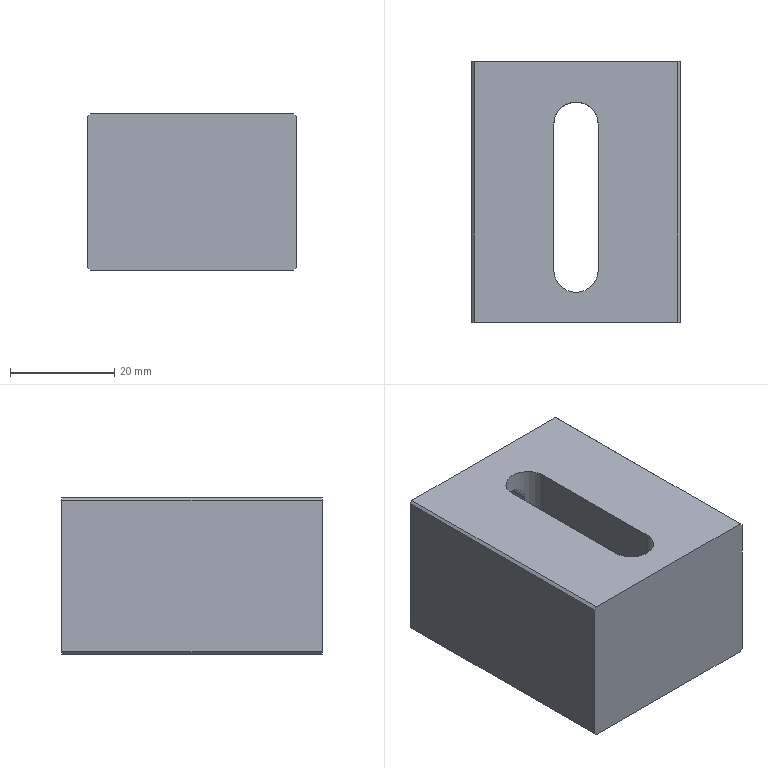Part | NX | 1 solid | 20 faces | box 40 x 50 x 30 mm | volume 50212 mm3 | plane 12 | cylinder 6 | cone 2 | commonest cylinder face diameters 5 x4 8.5 x2
STEP:
#1=CARTESIAN_POINT('',(-19.5,25.,0.));
#2=VERTEX_POINT('',#1);
#3=CARTESIAN_POINT('',(-20.,25.,0.5));
#4=VERTEX_POINT('',#3);
#5=CARTESIAN_POINT('',(-20.,25.,0.5));
#6=DIRECTION('',(-0.7071,0.,0.7071));
#7=VECTOR('',#6,1000.);
#8=LINE('',#5,#7);
#9=EDGE_CURVE('',#2,#4,#8,.T.);
#10=ORIENTED_EDGE('',*,*,#9,.F.);
#11=CARTESIAN_POINT('',(-19.5,-25.,0.));
#12=VERTEX_POINT('',#11);
#13=CARTESIAN_POINT('',(-19.5,0.,0.));
#14=DIRECTION('',(0.,1.,0.));
#15=VECTOR('',#14,1000.);
#16=LINE('',#13,#15);
#17=EDGE_CURVE('',#12,#2,#16,.T.);
#18=ORIENTED_EDGE('',*,*,#17,.F.);
#19=CARTESIAN_POINT('',(-20.,-25.,0.5));
#20=VERTEX_POINT('',#19);
#21=CARTESIAN_POINT('',(-20.,-25.,0.5));
#22=DIRECTION('',(0.7071,0.,-0.7071));
#23=VECTOR('',#22,1000.);
#24=LINE('',#21,#23);
#25=EDGE_CURVE('',#20,#12,#24,.T.);
#26=ORIENTED_EDGE('',*,*,#25,.F.);
#27=CARTESIAN_POINT('',(-20.,25.,0.5));
#28=DIRECTION('',(0.,-1.,0.));
#29=VECTOR('',#28,1000.);
#30=LINE('',#27,#29);
#31=EDGE_CURVE('',#4,#20,#30,.T.);
#32=ORIENTED_EDGE('',*,*,#31,.F.);
#33=EDGE_LOOP('',(#10,#18,#26,#32));
#34=FACE_BOUND('',#33,.T.);
#35=CARTESIAN_POINT('',(-20.,25.,0.5));
#36=DIRECTION('',(0.7071,0.,0.7071));
#37=DIRECTION('',(0.,-1.,0.));
#38=AXIS2_PLACEMENT_3D('',#35,#36,#37);
#39=PLANE('',#38);
#40=ADVANCED_FACE('',(#34),#39,.F.);
#41=CARTESIAN_POINT('',(-20.,25.,29.5));
#42=VERTEX_POINT('',#41);
#43=CARTESIAN_POINT('',(-19.5,25.,30.));
#44=VERTEX_POINT('',#43);
#45=CARTESIAN_POINT('',(-19.5,25.,30.));
#46=DIRECTION('',(0.7071,0.,0.7071));
#47=VECTOR('',#46,1000.);
#48=LINE('',#45,#47);
#49=EDGE_CURVE('',#42,#44,#48,.T.);
#50=ORIENTED_EDGE('',*,*,#49,.F.);
#51=CARTESIAN_POINT('',(-20.,-25.,29.5));
#52=VERTEX_POINT('',#51);
#53=CARTESIAN_POINT('',(-20.,25.,29.5));
#54=DIRECTION('',(0.,1.,0.));
#55=VECTOR('',#54,1000.);
#56=LINE('',#53,#55);
#57=EDGE_CURVE('',#52,#42,#56,.T.);
#58=ORIENTED_EDGE('',*,*,#57,.F.);
#59=CARTESIAN_POINT('',(-19.5,-25.,30.));
#60=VERTEX_POINT('',#59);
#61=CARTESIAN_POINT('',(-19.5,-25.,30.));
#62=DIRECTION('',(-0.7071,0.,-0.7071));
#63=VECTOR('',#62,1000.);
#64=LINE('',#61,#63);
#65=EDGE_CURVE('',#60,#52,#64,.T.);
#66=ORIENTED_EDGE('',*,*,#65,.F.);
#67=CARTESIAN_POINT('',(-19.5,-25.,30.));
#68=DIRECTION('',(0.,-1.,0.));
#69=VECTOR('',#68,1000.);
#70=LINE('',#67,#69);
#71=EDGE_CURVE('',#44,#60,#70,.T.);
#72=ORIENTED_EDGE('',*,*,#71,.F.);
#73=EDGE_LOOP('',(#50,#58,#66,#72));
#74=FACE_BOUND('',#73,.T.);
#75=CARTESIAN_POINT('',(-19.5,0.,30.));
#76=DIRECTION('',(-0.7071,0.,0.7071));
#77=DIRECTION('',(0.,1.,0.));
#78=AXIS2_PLACEMENT_3D('',#75,#76,#77);
#79=PLANE('',#78);
#80=ADVANCED_FACE('',(#74),#79,.T.);
#81=CARTESIAN_POINT('',(19.5,-25.,0.));
#82=VERTEX_POINT('',#81);
#83=CARTESIAN_POINT('',(20.,-25.,0.5));
#84=VERTEX_POINT('',#83);
#85=CARTESIAN_POINT('',(20.,-25.,0.5));
#86=DIRECTION('',(0.7071,0.,0.7071));
#87=VECTOR('',#86,1000.);
#88=LINE('',#85,#87);
#89=EDGE_CURVE('',#82,#84,#88,.T.);
#90=ORIENTED_EDGE('',*,*,#89,.F.);
#91=CARTESIAN_POINT('',(19.5,25.,0.));
#92=VERTEX_POINT('',#91);
#93=CARTESIAN_POINT('',(19.5,0.,0.));
#94=DIRECTION('',(0.,-1.,0.));
#95=VECTOR('',#94,1000.);
#96=LINE('',#93,#95);
#97=EDGE_CURVE('',#92,#82,#96,.T.);
#98=ORIENTED_EDGE('',*,*,#97,.F.);
#99=CARTESIAN_POINT('',(20.,25.,0.5));
#100=VERTEX_POINT('',#99);
#101=CARTESIAN_POINT('',(20.,25.,0.5));
#102=DIRECTION('',(-0.7071,0.,-0.7071));
#103=VECTOR('',#102,1000.);
#104=LINE('',#101,#103);
#105=EDGE_CURVE('',#100,#92,#104,.T.);
#106=ORIENTED_EDGE('',*,*,#105,.F.);
#107=CARTESIAN_POINT('',(20.,25.,0.5));
#108=DIRECTION('',(0.,1.,0.));
#109=VECTOR('',#108,1000.);
#110=LINE('',#107,#109);
#111=EDGE_CURVE('',#84,#100,#110,.T.);
#112=ORIENTED_EDGE('',*,*,#111,.F.);
#113=EDGE_LOOP('',(#90,#98,#106,#112));
#114=FACE_BOUND('',#113,.T.);
#115=CARTESIAN_POINT('',(20.,25.,0.5));
#116=DIRECTION('',(-0.7071,0.,0.7071));
#117=DIRECTION('',(0.,1.,0.));
#118=AXIS2_PLACEMENT_3D('',#115,#116,#117);
#119=PLANE('',#118);
#120=ADVANCED_FACE('',(#114),#119,.F.);
#121=CARTESIAN_POINT('',(20.,-25.,29.5));
#122=VERTEX_POINT('',#121);
#123=CARTESIAN_POINT('',(19.5,-25.,30.));
#124=VERTEX_POINT('',#123);
#125=CARTESIAN_POINT('',(19.5,-25.,30.));
#126=DIRECTION('',(-0.7071,0.,0.7071));
#127=VECTOR('',#126,1000.);
#128=LINE('',#125,#127);
#129=EDGE_CURVE('',#122,#124,#128,.T.);
#130=ORIENTED_EDGE('',*,*,#129,.F.);
#131=CARTESIAN_POINT('',(20.,25.,29.5));
#132=VERTEX_POINT('',#131);
#133=CARTESIAN_POINT('',(20.,-25.,29.5));
#134=DIRECTION('',(0.,-1.,0.));
#135=VECTOR('',#134,1000.);
#136=LINE('',#133,#135);
#137=EDGE_CURVE('',#132,#122,#136,.T.);
#138=ORIENTED_EDGE('',*,*,#137,.F.);
#139=CARTESIAN_POINT('',(19.5,25.,30.));
#140=VERTEX_POINT('',#139);
#141=CARTESIAN_POINT('',(19.5,25.,30.));
#142=DIRECTION('',(0.7071,0.,-0.7071));
#143=VECTOR('',#142,1000.);
#144=LINE('',#141,#143);
#145=EDGE_CURVE('',#140,#132,#144,.T.);
#146=ORIENTED_EDGE('',*,*,#145,.F.);
#147=CARTESIAN_POINT('',(19.5,25.,30.));
#148=DIRECTION('',(0.,1.,0.));
#149=VECTOR('',#148,1000.);
#150=LINE('',#147,#149);
#151=EDGE_CURVE('',#124,#140,#150,.T.);
#152=ORIENTED_EDGE('',*,*,#151,.F.);
#153=EDGE_LOOP('',(#130,#138,#146,#152));
#154=FACE_BOUND('',#153,.T.);
#155=CARTESIAN_POINT('',(19.5,0.,30.));
#156=DIRECTION('',(0.7071,0.,0.7071));
#157=DIRECTION('',(0.,-1.,0.));
#158=AXIS2_PLACEMENT_3D('',#155,#156,#157);
#159=PLANE('',#158);
#160=ADVANCED_FACE('',(#154),#159,.T.);
#161=CARTESIAN_POINT('',(-4.25,13.,30.));
#162=VERTEX_POINT('',#161);
#163=CARTESIAN_POINT('',(-4.25,-15.,30.));
#164=VERTEX_POINT('',#163);
#165=CARTESIAN_POINT('',(-4.25,13.,30.));
#166=DIRECTION('',(0.,-1.,0.));
#167=VECTOR('',#166,1000.);
#168=LINE('',#165,#167);
#169=EDGE_CURVE('',#162,#164,#168,.T.);
#170=ORIENTED_EDGE('',*,*,#169,.T.);
#171=CARTESIAN_POINT('',(-4.25,-15.,0.));
#172=VERTEX_POINT('',#171);
#173=CARTESIAN_POINT('',(-4.25,-15.,0.));
#174=DIRECTION('',(0.,0.,1.));
#175=VECTOR('',#174,1000.);
#176=LINE('',#173,#175);
#177=EDGE_CURVE('',#172,#164,#176,.T.);
#178=ORIENTED_EDGE('',*,*,#177,.F.);
#179=CARTESIAN_POINT('',(-4.25,13.,0.));
#180=VERTEX_POINT('',#179);
#181=CARTESIAN_POINT('',(-4.25,13.,0.));
#182=DIRECTION('',(0.,-1.,0.));
#183=VECTOR('',#182,1000.);
#184=LINE('',#181,#183);
#185=EDGE_CURVE('',#180,#172,#184,.T.);
#186=ORIENTED_EDGE('',*,*,#185,.F.);
#187=CARTESIAN_POINT('',(-4.25,13.,0.));
#188=DIRECTION('',(0.,0.,1.));
#189=VECTOR('',#188,1000.);
#190=LINE('',#187,#189);
#191=EDGE_CURVE('',#180,#162,#190,.T.);
#192=ORIENTED_EDGE('',*,*,#191,.T.);
#193=EDGE_LOOP('',(#170,#178,#186,#192));
#194=FACE_BOUND('',#193,.T.);
#195=CARTESIAN_POINT('',(-4.25,13.,0.));
#196=DIRECTION('',(-1.,0.,0.));
#197=DIRECTION('',(0.,-1.,0.));
#198=AXIS2_PLACEMENT_3D('',#195,#196,#197);
#199=PLANE('',#198);
#200=ADVANCED_FACE('',(#194),#199,.F.);
#201=CARTESIAN_POINT('',(4.25,-15.,30.));
#202=VERTEX_POINT('',#201);
#203=CARTESIAN_POINT('',(0.,-15.,30.));
#204=DIRECTION('',(0.,0.,1.));
#205=DIRECTION('',(1.,0.,0.));
#206=AXIS2_PLACEMENT_3D('',#203,#204,#205);
#207=CIRCLE('',#206,4.25);
#208=EDGE_CURVE('',#164,#202,#207,.T.);
#209=ORIENTED_EDGE('',*,*,#208,.T.);
#210=CARTESIAN_POINT('',(4.25,-15.,0.));
#211=VERTEX_POINT('',#210);
#212=CARTESIAN_POINT('',(4.25,-15.,0.));
#213=DIRECTION('',(0.,0.,1.));
#214=VECTOR('',#213,1000.);
#215=LINE('',#212,#214);
#216=EDGE_CURVE('',#211,#202,#215,.T.);
#217=ORIENTED_EDGE('',*,*,#216,.F.);
#218=CARTESIAN_POINT('',(0.,-15.,0.));
#219=DIRECTION('',(0.,0.,1.));
#220=DIRECTION('',(1.,0.,0.));
#221=AXIS2_PLACEMENT_3D('',#218,#219,#220);
#222=CIRCLE('',#221,4.25);
#223=EDGE_CURVE('',#172,#211,#222,.T.);
#224=ORIENTED_EDGE('',*,*,#223,.F.);
#225=ORIENTED_EDGE('',*,*,#177,.T.);
#226=EDGE_LOOP('',(#209,#217,#224,#225));
#227=FACE_BOUND('',#226,.T.);
#228=CARTESIAN_POINT('',(0.,-15.,0.));
#229=DIRECTION('',(0.,0.,1.));
#230=DIRECTION('',(1.,0.,0.));
#231=AXIS2_PLACEMENT_3D('',#228,#229,#230);
#232=CYLINDRICAL_SURFACE('',#231,4.25);
#233=ADVANCED_FACE('',(#227),#232,.F.);
#234=CARTESIAN_POINT('',(4.25,13.,30.));
#235=VERTEX_POINT('',#234);
#236=CARTESIAN_POINT('',(4.25,13.,30.));
#237=DIRECTION('',(0.,1.,0.));
#238=VECTOR('',#237,1000.);
#239=LINE('',#236,#238);
#240=EDGE_CURVE('',#202,#235,#239,.T.);
#241=ORIENTED_EDGE('',*,*,#240,.T.);
#242=CARTESIAN_POINT('',(4.25,13.,0.));
#243=VERTEX_POINT('',#242);
#244=CARTESIAN_POINT('',(4.25,13.,0.));
#245=DIRECTION('',(0.,0.,1.));
#246=VECTOR('',#245,1000.);
#247=LINE('',#244,#246);
#248=EDGE_CURVE('',#243,#235,#247,.T.);
#249=ORIENTED_EDGE('',*,*,#248,.F.);
#250=CARTESIAN_POINT('',(4.25,13.,0.));
#251=DIRECTION('',(0.,1.,0.));
#252=VECTOR('',#251,1000.);
#253=LINE('',#250,#252);
#254=EDGE_CURVE('',#211,#243,#253,.T.);
#255=ORIENTED_EDGE('',*,*,#254,.F.);
#256=ORIENTED_EDGE('',*,*,#216,.T.);
#257=EDGE_LOOP('',(#241,#249,#255,#256));
#258=FACE_BOUND('',#257,.T.);
#259=CARTESIAN_POINT('',(4.25,13.,0.));
#260=DIRECTION('',(1.,0.,0.));
#261=DIRECTION('',(0.,1.,0.));
#262=AXIS2_PLACEMENT_3D('',#259,#260,#261);
#263=PLANE('',#262);
#264=ADVANCED_FACE('',(#258),#263,.F.);
#265=CARTESIAN_POINT('',(0.,13.,30.));
#266=DIRECTION('',(0.,0.,1.));
#267=DIRECTION('',(1.,0.,0.));
#268=AXIS2_PLACEMENT_3D('',#265,#266,#267);
#269=CIRCLE('',#268,4.25);
#270=EDGE_CURVE('',#235,#162,#269,.T.);
#271=ORIENTED_EDGE('',*,*,#270,.T.);
#272=ORIENTED_EDGE('',*,*,#191,.F.);
#273=CARTESIAN_POINT('',(0.,13.,0.));
#274=DIRECTION('',(0.,0.,1.));
#275=DIRECTION('',(1.,0.,0.));
#276=AXIS2_PLACEMENT_3D('',#273,#274,#275);
#277=CIRCLE('',#276,4.25);
#278=EDGE_CURVE('',#243,#180,#277,.T.);
#279=ORIENTED_EDGE('',*,*,#278,.F.);
#280=ORIENTED_EDGE('',*,*,#248,.T.);
#281=EDGE_LOOP('',(#271,#272,#279,#280));
#282=FACE_BOUND('',#281,.T.);
#283=CARTESIAN_POINT('',(0.,17.25,21.5));
#284=VERTEX_POINT('',#283);
#285=CARTESIAN_POINT('',(1.967,16.883,22.047));
#286=CARTESIAN_POINT('',(-0.001371,17.433,21.227));
#287=CARTESIAN_POINT('',(-1.961,16.885,22.045));
#288=CARTESIAN_POINT('',(-2.768,16.214,23.993));
#289=CARTESIAN_POINT('',(-1.968,16.881,25.95));
#290=CARTESIAN_POINT('',(-0.006057,17.433,26.773));
#291=CARTESIAN_POINT('',(1.961,16.886,25.957));
#292=CARTESIAN_POINT('',(2.768,16.213,24.007));
#293=CARTESIAN_POINT('',(1.967,16.883,22.047));
#294=CARTESIAN_POINT('',(-0.001371,17.433,21.227));
#295=CARTESIAN_POINT('',(-1.961,16.885,22.045));
#296=B_SPLINE_CURVE_WITH_KNOTS('',3,(#285,#286,#287,#288,#289,#290,#291,#292,#293,#294,#295),.UNSPECIFIED.,.T.,.F.,(1,1,1,1,1,1,1,1,1,1,1,1,1,1,1),(-0.006002,-0.004001,-0.002001,0.,0.002001,0.004001,0.006002,0.008002,0.01,0.012,0.014,0.016,0.01801,0.02001,0.02201),.UNSPECIFIED.);
#297=EDGE_CURVE('',#284,#284,#296,.T.);
#298=ORIENTED_EDGE('',*,*,#297,.T.);
#299=EDGE_LOOP('',(#298));
#300=FACE_BOUND('',#299,.T.);
#301=CARTESIAN_POINT('',(0.,17.25,3.5));
#302=VERTEX_POINT('',#301);
#303=CARTESIAN_POINT('',(1.967,16.883,4.047));
#304=CARTESIAN_POINT('',(-0.001371,17.433,3.227));
#305=CARTESIAN_POINT('',(-1.961,16.885,4.045));
#306=CARTESIAN_POINT('',(-2.768,16.214,5.993));
#307=CARTESIAN_POINT('',(-1.968,16.881,7.95));
#308=CARTESIAN_POINT('',(-0.006057,17.433,8.773));
#309=CARTESIAN_POINT('',(1.961,16.886,7.957));
#310=CARTESIAN_POINT('',(2.768,16.213,6.007));
#311=CARTESIAN_POINT('',(1.967,16.883,4.047));
#312=CARTESIAN_POINT('',(-0.001371,17.433,3.227));
#313=CARTESIAN_POINT('',(-1.961,16.885,4.045));
#314=B_SPLINE_CURVE_WITH_KNOTS('',3,(#303,#304,#305,#306,#307,#308,#309,#310,#311,#312,#313),.UNSPECIFIED.,.T.,.F.,(1,1,1,1,1,1,1,1,1,1,1,1,1,1,1),(-0.006002,-0.004001,-0.002001,0.,0.002001,0.004001,0.006002,0.008002,0.01,0.012,0.014,0.016,0.01801,0.02001,0.02201),.UNSPECIFIED.);
#315=EDGE_CURVE('',#302,#302,#314,.T.);
#316=ORIENTED_EDGE('',*,*,#315,.T.);
#317=EDGE_LOOP('',(#316));
#318=FACE_BOUND('',#317,.T.);
#319=CARTESIAN_POINT('',(0.,13.,0.));
#320=DIRECTION('',(0.,0.,1.));
#321=DIRECTION('',(1.,0.,0.));
#322=AXIS2_PLACEMENT_3D('',#319,#320,#321);
#323=CYLINDRICAL_SURFACE('',#322,4.25);
#324=ADVANCED_FACE('',(#282,#300,#318),#323,.F.);
#325=CARTESIAN_POINT('',(-20.,25.,0.));
#326=DIRECTION('',(-1.,0.,0.));
#327=VECTOR('',#326,1000.);
#328=LINE('',#325,#327);
#329=EDGE_CURVE('',#92,#2,#328,.T.);
#330=ORIENTED_EDGE('',*,*,#329,.F.);
#331=ORIENTED_EDGE('',*,*,#97,.T.);
#332=CARTESIAN_POINT('',(-20.,-25.,0.));
#333=DIRECTION('',(1.,0.,0.));
#334=VECTOR('',#333,1000.);
#335=LINE('',#332,#334);
#336=EDGE_CURVE('',#12,#82,#335,.T.);
#337=ORIENTED_EDGE('',*,*,#336,.F.);
#338=ORIENTED_EDGE('',*,*,#17,.T.);
#339=EDGE_LOOP('',(#330,#331,#337,#338));
#340=FACE_BOUND('',#339,.T.);
#341=ORIENTED_EDGE('',*,*,#254,.T.);
#342=ORIENTED_EDGE('',*,*,#278,.T.);
#343=ORIENTED_EDGE('',*,*,#185,.T.);
#344=ORIENTED_EDGE('',*,*,#223,.T.);
#345=EDGE_LOOP('',(#341,#342,#343,#344));
#346=FACE_BOUND('',#345,.T.);
#347=CARTESIAN_POINT('',(0.,0.,0.));
#348=DIRECTION('',(0.,0.,1.));
#349=DIRECTION('',(1.,0.,0.));
#350=AXIS2_PLACEMENT_3D('',#347,#348,#349);
#351=PLANE('',#350);
#352=ADVANCED_FACE('',(#340,#346),#351,.F.);
#353=CARTESIAN_POINT('',(-20.,-25.,30.));
#354=DIRECTION('',(1.,0.,0.));
#355=VECTOR('',#354,1000.);
#356=LINE('',#353,#355);
#357=EDGE_CURVE('',#60,#124,#356,.T.);
#358=ORIENTED_EDGE('',*,*,#357,.T.);
#359=ORIENTED_EDGE('',*,*,#151,.T.);
#360=CARTESIAN_POINT('',(-20.,25.,30.));
#361=DIRECTION('',(-1.,0.,0.));
#362=VECTOR('',#361,1000.);
#363=LINE('',#360,#362);
#364=EDGE_CURVE('',#140,#44,#363,.T.);
#365=ORIENTED_EDGE('',*,*,#364,.T.);
#366=ORIENTED_EDGE('',*,*,#71,.T.);
#367=EDGE_LOOP('',(#358,#359,#365,#366));
#368=FACE_BOUND('',#367,.T.);
#369=ORIENTED_EDGE('',*,*,#270,.F.);
#370=ORIENTED_EDGE('',*,*,#240,.F.);
#371=ORIENTED_EDGE('',*,*,#208,.F.);
#372=ORIENTED_EDGE('',*,*,#169,.F.);
#373=EDGE_LOOP('',(#369,#370,#371,#372));
#374=FACE_BOUND('',#373,.T.);
#375=CARTESIAN_POINT('',(0.,0.,30.));
#376=DIRECTION('',(0.,0.,1.));
#377=DIRECTION('',(1.,0.,0.));
#378=AXIS2_PLACEMENT_3D('',#375,#376,#377);
#379=PLANE('',#378);
#380=ADVANCED_FACE('',(#368,#374),#379,.T.);
#381=CARTESIAN_POINT('',(20.,-25.,30.));
#382=DIRECTION('',(0.,0.,-1.));
#383=VECTOR('',#382,1000.);
#384=LINE('',#381,#383);
#385=EDGE_CURVE('',#122,#84,#384,.T.);
#386=ORIENTED_EDGE('',*,*,#385,.F.);
#387=ORIENTED_EDGE('',*,*,#129,.T.);
#388=ORIENTED_EDGE('',*,*,#357,.F.);
#389=ORIENTED_EDGE('',*,*,#65,.T.);
#390=CARTESIAN_POINT('',(-20.,-25.,30.));
#391=DIRECTION('',(0.,0.,-1.));
#392=VECTOR('',#391,1000.);
#393=LINE('',#390,#392);
#394=EDGE_CURVE('',#52,#20,#393,.T.);
#395=ORIENTED_EDGE('',*,*,#394,.T.);
#396=ORIENTED_EDGE('',*,*,#25,.T.);
#397=ORIENTED_EDGE('',*,*,#336,.T.);
#398=ORIENTED_EDGE('',*,*,#89,.T.);
#399=EDGE_LOOP('',(#386,#387,#388,#389,#395,#396,#397,#398));
#400=FACE_BOUND('',#399,.T.);
#401=CARTESIAN_POINT('',(-20.,-25.,30.));
#402=DIRECTION('',(0.,1.,0.));
#403=DIRECTION('',(0.,0.,1.));
#404=AXIS2_PLACEMENT_3D('',#401,#402,#403);
#405=PLANE('',#404);
#406=ADVANCED_FACE('',(#400),#405,.F.);
#407=ORIENTED_EDGE('',*,*,#394,.F.);
#408=ORIENTED_EDGE('',*,*,#57,.T.);
#409=CARTESIAN_POINT('',(-20.,25.,30.));
#410=DIRECTION('',(0.,0.,-1.));
#411=VECTOR('',#410,1000.);
#412=LINE('',#409,#411);
#413=EDGE_CURVE('',#42,#4,#412,.T.);
#414=ORIENTED_EDGE('',*,*,#413,.T.);
#415=ORIENTED_EDGE('',*,*,#31,.T.);
#416=EDGE_LOOP('',(#407,#408,#414,#415));
#417=FACE_BOUND('',#416,.T.);
#418=CARTESIAN_POINT('',(-20.,25.,30.));
#419=DIRECTION('',(1.,0.,0.));
#420=DIRECTION('',(0.,1.,0.));
#421=AXIS2_PLACEMENT_3D('',#418,#419,#420);
#422=PLANE('',#421);
#423=ADVANCED_FACE('',(#417),#422,.F.);
#424=ORIENTED_EDGE('',*,*,#364,.F.);
#425=ORIENTED_EDGE('',*,*,#145,.T.);
#426=CARTESIAN_POINT('',(20.,25.,30.));
#427=DIRECTION('',(0.,0.,-1.));
#428=VECTOR('',#427,1000.);
#429=LINE('',#426,#428);
#430=EDGE_CURVE('',#132,#100,#429,.T.);
#431=ORIENTED_EDGE('',*,*,#430,.T.);
#432=ORIENTED_EDGE('',*,*,#105,.T.);
#433=ORIENTED_EDGE('',*,*,#329,.T.);
#434=ORIENTED_EDGE('',*,*,#9,.T.);
#435=ORIENTED_EDGE('',*,*,#413,.F.);
#436=ORIENTED_EDGE('',*,*,#49,.T.);
#437=EDGE_LOOP('',(#424,#425,#431,#432,#433,#434,#435,#436));
#438=FACE_BOUND('',#437,.T.);
#439=CARTESIAN_POINT('',(-12.,25.,17.5));
#440=VERTEX_POINT('',#439);
#441=CARTESIAN_POINT('',(-12.,25.,15.));
#442=DIRECTION('',(0.,1.,0.));
#443=DIRECTION('',(0.,0.,1.));
#444=AXIS2_PLACEMENT_3D('',#441,#442,#443);
#445=CIRCLE('',#444,2.5);
#446=EDGE_CURVE('',#440,#440,#445,.T.);
#447=ORIENTED_EDGE('',*,*,#446,.F.);
#448=EDGE_LOOP('',(#447));
#449=FACE_BOUND('',#448,.T.);
#450=CARTESIAN_POINT('',(12.,25.,17.5));
#451=VERTEX_POINT('',#450);
#452=CARTESIAN_POINT('',(12.,25.,15.));
#453=DIRECTION('',(0.,1.,0.));
#454=DIRECTION('',(0.,0.,1.));
#455=AXIS2_PLACEMENT_3D('',#452,#453,#454);
#456=CIRCLE('',#455,2.5);
#457=EDGE_CURVE('',#451,#451,#456,.T.);
#458=ORIENTED_EDGE('',*,*,#457,.F.);
#459=EDGE_LOOP('',(#458));
#460=FACE_BOUND('',#459,.T.);
#461=CARTESIAN_POINT('',(0.,25.,26.5));
#462=VERTEX_POINT('',#461);
#463=CARTESIAN_POINT('',(0.,25.,24.));
#464=DIRECTION('',(0.,1.,0.));
#465=DIRECTION('',(0.,0.,1.));
#466=AXIS2_PLACEMENT_3D('',#463,#464,#465);
#467=CIRCLE('',#466,2.5);
#468=EDGE_CURVE('',#462,#462,#467,.T.);
#469=ORIENTED_EDGE('',*,*,#468,.F.);
#470=EDGE_LOOP('',(#469));
#471=FACE_BOUND('',#470,.T.);
#472=CARTESIAN_POINT('',(0.,25.,8.5));
#473=VERTEX_POINT('',#472);
#474=CARTESIAN_POINT('',(0.,25.,6.));
#475=DIRECTION('',(0.,1.,0.));
#476=DIRECTION('',(0.,0.,1.));
#477=AXIS2_PLACEMENT_3D('',#474,#475,#476);
#478=CIRCLE('',#477,2.5);
#479=EDGE_CURVE('',#473,#473,#478,.T.);
#480=ORIENTED_EDGE('',*,*,#479,.F.);
#481=EDGE_LOOP('',(#480));
#482=FACE_BOUND('',#481,.T.);
#483=CARTESIAN_POINT('',(-20.,25.,30.));
#484=DIRECTION('',(0.,-1.,0.));
#485=DIRECTION('',(0.,0.,-1.));
#486=AXIS2_PLACEMENT_3D('',#483,#484,#485);
#487=PLANE('',#486);
#488=ADVANCED_FACE('',(#438,#449,#460,#471,#482),#487,.F.);
#489=ORIENTED_EDGE('',*,*,#430,.F.);
#490=ORIENTED_EDGE('',*,*,#137,.T.);
#491=ORIENTED_EDGE('',*,*,#385,.T.);
#492=ORIENTED_EDGE('',*,*,#111,.T.);
#493=EDGE_LOOP('',(#489,#490,#491,#492));
#494=FACE_BOUND('',#493,.T.);
#495=CARTESIAN_POINT('',(20.,25.,30.));
#496=DIRECTION('',(-1.,0.,0.));
#497=DIRECTION('',(0.,-1.,0.));
#498=AXIS2_PLACEMENT_3D('',#495,#496,#497);
#499=PLANE('',#498);
#500=ADVANCED_FACE('',(#494),#499,.F.);
#501=CARTESIAN_POINT('',(-12.,10.,17.5));
#502=VERTEX_POINT('',#501);
#503=CARTESIAN_POINT('',(-12.,10.,15.));
#504=DIRECTION('',(0.,1.,0.));
#505=DIRECTION('',(0.,0.,1.));
#506=AXIS2_PLACEMENT_3D('',#503,#504,#505);
#507=CIRCLE('',#506,2.5);
#508=EDGE_CURVE('',#502,#502,#507,.T.);
#509=ORIENTED_EDGE('',*,*,#508,.T.);
#510=EDGE_LOOP('',(#509));
#511=FACE_BOUND('',#510,.T.);
#512=CARTESIAN_POINT('',(-12.,8.498,15.));
#513=VERTEX_POINT('',#512);
#514=VERTEX_LOOP('',#513);
#515=FACE_BOUND('',#514,.T.);
#516=CARTESIAN_POINT('',(-12.,10.,15.));
#517=DIRECTION('',(0.,1.,0.));
#518=DIRECTION('',(0.,0.,1.));
#519=AXIS2_PLACEMENT_3D('',#516,#517,#518);
#520=CONICAL_SURFACE('',#519,2.5,1.03);
#521=ADVANCED_FACE('',(#511,#515),#520,.F.);
#522=ORIENTED_EDGE('',*,*,#508,.F.);
#523=EDGE_LOOP('',(#522));
#524=FACE_BOUND('',#523,.T.);
#525=ORIENTED_EDGE('',*,*,#446,.T.);
#526=EDGE_LOOP('',(#525));
#527=FACE_BOUND('',#526,.T.);
#528=CARTESIAN_POINT('',(-12.,25.,15.));
#529=DIRECTION('',(0.,1.,0.));
#530=DIRECTION('',(0.,0.,1.));
#531=AXIS2_PLACEMENT_3D('',#528,#529,#530);
#532=CYLINDRICAL_SURFACE('',#531,2.5);
#533=ADVANCED_FACE('',(#524,#527),#532,.F.);
#534=CARTESIAN_POINT('',(12.,10.,17.5));
#535=VERTEX_POINT('',#534);
#536=CARTESIAN_POINT('',(12.,10.,15.));
#537=DIRECTION('',(0.,1.,0.));
#538=DIRECTION('',(0.,0.,1.));
#539=AXIS2_PLACEMENT_3D('',#536,#537,#538);
#540=CIRCLE('',#539,2.5);
#541=EDGE_CURVE('',#535,#535,#540,.T.);
#542=ORIENTED_EDGE('',*,*,#541,.T.);
#543=EDGE_LOOP('',(#542));
#544=FACE_BOUND('',#543,.T.);
#545=CARTESIAN_POINT('',(12.,8.498,15.));
#546=VERTEX_POINT('',#545);
#547=VERTEX_LOOP('',#546);
#548=FACE_BOUND('',#547,.T.);
#549=CARTESIAN_POINT('',(12.,10.,15.));
#550=DIRECTION('',(0.,1.,0.));
#551=DIRECTION('',(0.,0.,1.));
#552=AXIS2_PLACEMENT_3D('',#549,#550,#551);
#553=CONICAL_SURFACE('',#552,2.5,1.03);
#554=ADVANCED_FACE('',(#544,#548),#553,.F.);
#555=ORIENTED_EDGE('',*,*,#541,.F.);
#556=EDGE_LOOP('',(#555));
#557=FACE_BOUND('',#556,.T.);
#558=ORIENTED_EDGE('',*,*,#457,.T.);
#559=EDGE_LOOP('',(#558));
#560=FACE_BOUND('',#559,.T.);
#561=CARTESIAN_POINT('',(12.,25.,15.));
#562=DIRECTION('',(0.,1.,0.));
#563=DIRECTION('',(0.,0.,1.));
#564=AXIS2_PLACEMENT_3D('',#561,#562,#563);
#565=CYLINDRICAL_SURFACE('',#564,2.5);
#566=ADVANCED_FACE('',(#557,#560),#565,.F.);
#567=ORIENTED_EDGE('',*,*,#297,.F.);
#568=EDGE_LOOP('',(#567));
#569=FACE_BOUND('',#568,.T.);
#570=ORIENTED_EDGE('',*,*,#468,.T.);
#571=EDGE_LOOP('',(#570));
#572=FACE_BOUND('',#571,.T.);
#573=CARTESIAN_POINT('',(0.,25.,24.));
#574=DIRECTION('',(0.,1.,0.));
#575=DIRECTION('',(0.,0.,1.));
#576=AXIS2_PLACEMENT_3D('',#573,#574,#575);
#577=CYLINDRICAL_SURFACE('',#576,2.5);
#578=ADVANCED_FACE('',(#569,#572),#577,.F.);
#579=ORIENTED_EDGE('',*,*,#315,.F.);
#580=EDGE_LOOP('',(#579));
#581=FACE_BOUND('',#580,.T.);
#582=ORIENTED_EDGE('',*,*,#479,.T.);
#583=EDGE_LOOP('',(#582));
#584=FACE_BOUND('',#583,.T.);
#585=CARTESIAN_POINT('',(0.,25.,6.));
#586=DIRECTION('',(0.,1.,0.));
#587=DIRECTION('',(0.,0.,1.));
#588=AXIS2_PLACEMENT_3D('',#585,#586,#587);
#589=CYLINDRICAL_SURFACE('',#588,2.5);
#590=ADVANCED_FACE('',(#581,#584),#589,.F.);
#591=CLOSED_SHELL('',(#40,#80,#120,#160,#200,#233,#264,#324,#352,#380,#406,#423,#488,#500,#521,#533,#554,#566,#578,#590));
#592=MANIFOLD_SOLID_BREP('',#591);
#593=(LENGTH_UNIT()NAMED_UNIT(*)SI_UNIT(.MILLI.,.METRE.));
#594=UNCERTAINTY_MEASURE_WITH_UNIT(LENGTH_MEASURE(0.0508),#593,'','');
#595=(NAMED_UNIT(*)PLANE_ANGLE_UNIT()SI_UNIT($,.RADIAN.));
#596=(NAMED_UNIT(*)SI_UNIT($,.STERADIAN.)SOLID_ANGLE_UNIT());
#597=(GEOMETRIC_REPRESENTATION_CONTEXT(3)GLOBAL_UNCERTAINTY_ASSIGNED_CONTEXT((#594))GLOBAL_UNIT_ASSIGNED_CONTEXT((#593,#595,#596))REPRESENTATION_CONTEXT('',''));
#598=ADVANCED_BREP_SHAPE_REPRESENTATION('',(#592),#597);